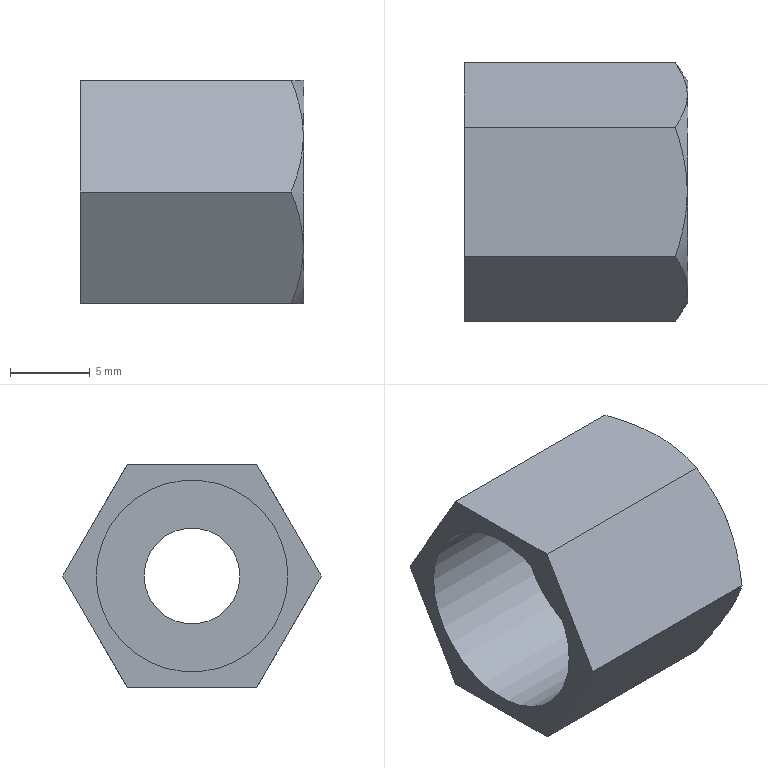Part | STEP file | 1-46.8 | 2 solids | 16 faces | box 14 x 16.166 x 14 mm | volume 1298 mm3 | plane 11 | cylinder 4 | cone 1 | commonest cylinder face diameters 6 x2 12 x2
STEP:
#1=CARTESIAN_POINT('',(0.,0.,0.));
#2=DIRECTION('',(0.,0.,1.));
#3=DIRECTION('',(1.,0.,0.));
#4=AXIS2_PLACEMENT_3D('',#1,#2,#3);
#5=CARTESIAN_POINT('',(11.,6.,0.));
#6=VERTEX_POINT('',#5);
#7=CARTESIAN_POINT('',(11.,0.,0.));
#8=DIRECTION('',(1.,0.,0.));
#9=DIRECTION('',(0.,1.,0.));
#10=AXIS2_PLACEMENT_3D('',#7,#8,#9);
#11=CIRCLE('',#10,6.);
#12=CARTESIAN_POINT('',(11.,-1.608,0.));
#13=DIRECTION('',(1.,0.,0.));
#14=DIRECTION('',(0.,0.,-1.));
#15=AXIS2_PLACEMENT_3D('',#12,#13,#14);
#16=PLANE('',#15);
#17=CARTESIAN_POINT('',(0.,1.608));
#18=DIRECTION('',(0.,1.));
#19=AXIS2_PLACEMENT_2D('',#17,#18);
#20=CIRCLE('',#19,6.);
#21=(GEOMETRIC_REPRESENTATION_CONTEXT(2)PARAMETRIC_REPRESENTATION_CONTEXT()REPRESENTATION_CONTEXT('',''));
#22=DEFINITIONAL_REPRESENTATION('',(#20),#21);
#23=PCURVE('',#16,#22);
#24=CARTESIAN_POINT('',(11.,0.,0.));
#25=DIRECTION('',(-1.,0.,0.));
#26=DIRECTION('',(0.,1.,0.));
#27=AXIS2_PLACEMENT_3D('',#24,#25,#26);
#28=CYLINDRICAL_SURFACE('',#27,6.);
#29=CARTESIAN_POINT('',(6.283,0.));
#30=DIRECTION('',(-1.,0.));
#31=VECTOR('',#30,1.);
#32=LINE('',#29,#31);
#33=(GEOMETRIC_REPRESENTATION_CONTEXT(2)PARAMETRIC_REPRESENTATION_CONTEXT()REPRESENTATION_CONTEXT('',''));
#34=DEFINITIONAL_REPRESENTATION('',(#32),#33);
#35=PCURVE('',#28,#34);
#36=SURFACE_CURVE('',#11,(#23,#35),.PCURVE_S1.);
#37=EDGE_CURVE('',#6,#6,#36,.T.);
#38=ORIENTED_EDGE('',*,*,#37,.T.);
#39=EDGE_LOOP('',(#38));
#40=FACE_BOUND('',#39,.T.);
#41=CARTESIAN_POINT('',(11.,3.,0.));
#42=VERTEX_POINT('',#41);
#43=CARTESIAN_POINT('',(11.,0.,0.));
#44=DIRECTION('',(-1.,0.,0.));
#45=DIRECTION('',(0.,1.,0.));
#46=AXIS2_PLACEMENT_3D('',#43,#44,#45);
#47=CIRCLE('',#46,3.);
#48=CARTESIAN_POINT('',(0.,4.608));
#49=CARTESIAN_POINT('',(5.196,4.608));
#50=CARTESIAN_POINT('',(2.598,0.1077));
#51=CARTESIAN_POINT('',(0.,-4.392));
#52=CARTESIAN_POINT('',(-2.598,0.1077));
#53=CARTESIAN_POINT('',(-5.196,4.608));
#54=CARTESIAN_POINT('',(0.,4.608));
#55=(BOUNDED_CURVE()B_SPLINE_CURVE(2,(#48,#49,#50,#51,#52,#53,#54),.UNSPECIFIED.,.T.,.F.)B_SPLINE_CURVE_WITH_KNOTS((1,2,2,2,2,1),(-2.094,0.,2.094,4.189,6.283,8.378),.UNSPECIFIED.)CURVE()GEOMETRIC_REPRESENTATION_ITEM()RATIONAL_B_SPLINE_CURVE((1.,0.5,1.,0.5,1.,0.5,1.))REPRESENTATION_ITEM(''));
#56=(GEOMETRIC_REPRESENTATION_CONTEXT(2)PARAMETRIC_REPRESENTATION_CONTEXT()REPRESENTATION_CONTEXT('',''));
#57=DEFINITIONAL_REPRESENTATION('',(#55),#56);
#58=PCURVE('',#16,#57);
#59=CARTESIAN_POINT('',(11.,0.,0.));
#60=DIRECTION('',(-1.,0.,0.));
#61=DIRECTION('',(0.,1.,0.));
#62=AXIS2_PLACEMENT_3D('',#59,#60,#61);
#63=CYLINDRICAL_SURFACE('',#62,3.);
#64=CARTESIAN_POINT('',(0.,0.));
#65=DIRECTION('',(1.,0.));
#66=VECTOR('',#65,1.);
#67=LINE('',#64,#66);
#68=(GEOMETRIC_REPRESENTATION_CONTEXT(2)PARAMETRIC_REPRESENTATION_CONTEXT()REPRESENTATION_CONTEXT('',''));
#69=DEFINITIONAL_REPRESENTATION('',(#67),#68);
#70=PCURVE('',#63,#69);
#71=SURFACE_CURVE('',#47,(#58,#70),.PCURVE_S1.);
#72=EDGE_CURVE('',#42,#42,#71,.T.);
#73=ORIENTED_EDGE('',*,*,#72,.T.);
#74=EDGE_LOOP('',(#73));
#75=FACE_BOUND('',#74,.T.);
#76=ADVANCED_FACE('',(#40,#75),#16,.T.);
#77=CARTESIAN_POINT('',(8.,6.,0.));
#78=VERTEX_POINT('',#77);
#79=CARTESIAN_POINT('',(8.,0.,0.));
#80=DIRECTION('',(1.,0.,0.));
#81=DIRECTION('',(0.,1.,0.));
#82=AXIS2_PLACEMENT_3D('',#79,#80,#81);
#83=CIRCLE('',#82,6.);
#84=CARTESIAN_POINT('',(8.,-1.608,0.));
#85=DIRECTION('',(1.,0.,0.));
#86=DIRECTION('',(0.,0.,-1.));
#87=AXIS2_PLACEMENT_3D('',#84,#85,#86);
#88=PLANE('',#87);
#89=CARTESIAN_POINT('',(0.,1.608));
#90=DIRECTION('',(0.,1.));
#91=AXIS2_PLACEMENT_2D('',#89,#90);
#92=CIRCLE('',#91,6.);
#93=(GEOMETRIC_REPRESENTATION_CONTEXT(2)PARAMETRIC_REPRESENTATION_CONTEXT()REPRESENTATION_CONTEXT('',''));
#94=DEFINITIONAL_REPRESENTATION('',(#92),#93);
#95=PCURVE('',#88,#94);
#96=CARTESIAN_POINT('',(6.283,3.));
#97=DIRECTION('',(-1.,0.));
#98=VECTOR('',#97,1.);
#99=LINE('',#96,#98);
#100=(GEOMETRIC_REPRESENTATION_CONTEXT(2)PARAMETRIC_REPRESENTATION_CONTEXT()REPRESENTATION_CONTEXT('',''));
#101=DEFINITIONAL_REPRESENTATION('',(#99),#100);
#102=PCURVE('',#28,#101);
#103=SURFACE_CURVE('',#83,(#95,#102),.PCURVE_S1.);
#104=EDGE_CURVE('',#78,#78,#103,.T.);
#105=ORIENTED_EDGE('',*,*,#104,.T.);
#106=EDGE_LOOP('',(#105));
#107=FACE_BOUND('',#106,.F.);
#108=CARTESIAN_POINT('',(8.,3.,0.));
#109=VERTEX_POINT('',#108);
#110=CARTESIAN_POINT('',(8.,0.,0.));
#111=DIRECTION('',(-1.,0.,0.));
#112=DIRECTION('',(0.,1.,0.));
#113=AXIS2_PLACEMENT_3D('',#110,#111,#112);
#114=CIRCLE('',#113,3.);
#115=CARTESIAN_POINT('',(0.,4.608));
#116=CARTESIAN_POINT('',(5.196,4.608));
#117=CARTESIAN_POINT('',(2.598,0.1077));
#118=CARTESIAN_POINT('',(0.,-4.392));
#119=CARTESIAN_POINT('',(-2.598,0.1077));
#120=CARTESIAN_POINT('',(-5.196,4.608));
#121=CARTESIAN_POINT('',(0.,4.608));
#122=(BOUNDED_CURVE()B_SPLINE_CURVE(2,(#115,#116,#117,#118,#119,#120,#121),.UNSPECIFIED.,.T.,.F.)B_SPLINE_CURVE_WITH_KNOTS((1,2,2,2,2,1),(-2.094,0.,2.094,4.189,6.283,8.378),.UNSPECIFIED.)CURVE()GEOMETRIC_REPRESENTATION_ITEM()RATIONAL_B_SPLINE_CURVE((1.,0.5,1.,0.5,1.,0.5,1.))REPRESENTATION_ITEM(''));
#123=(GEOMETRIC_REPRESENTATION_CONTEXT(2)PARAMETRIC_REPRESENTATION_CONTEXT()REPRESENTATION_CONTEXT('',''));
#124=DEFINITIONAL_REPRESENTATION('',(#122),#123);
#125=PCURVE('',#88,#124);
#126=CARTESIAN_POINT('',(0.,3.));
#127=DIRECTION('',(1.,0.));
#128=VECTOR('',#127,1.);
#129=LINE('',#126,#128);
#130=(GEOMETRIC_REPRESENTATION_CONTEXT(2)PARAMETRIC_REPRESENTATION_CONTEXT()REPRESENTATION_CONTEXT('',''));
#131=DEFINITIONAL_REPRESENTATION('',(#129),#130);
#132=PCURVE('',#63,#131);
#133=SURFACE_CURVE('',#114,(#125,#132),.PCURVE_S1.);
#134=EDGE_CURVE('',#109,#109,#133,.T.);
#135=ORIENTED_EDGE('',*,*,#134,.T.);
#136=EDGE_LOOP('',(#135));
#137=FACE_BOUND('',#136,.F.);
#138=ADVANCED_FACE('',(#107,#137),#88,.F.);
#139=CARTESIAN_POINT('',(11.,6.,0.));
#140=DIRECTION('',(-1.,0.,0.));
#141=VECTOR('',#140,1.);
#142=LINE('',#139,#141);
#143=CARTESIAN_POINT('',(6.283,0.));
#144=DIRECTION('',(0.,1.));
#145=VECTOR('',#144,1.);
#146=LINE('',#143,#145);
#147=(GEOMETRIC_REPRESENTATION_CONTEXT(2)PARAMETRIC_REPRESENTATION_CONTEXT()REPRESENTATION_CONTEXT('',''));
#148=DEFINITIONAL_REPRESENTATION('',(#146),#147);
#149=PCURVE('',#28,#148);
#150=CARTESIAN_POINT('',(0.,0.));
#151=DIRECTION('',(0.,1.));
#152=VECTOR('',#151,1.);
#153=LINE('',#150,#152);
#154=(GEOMETRIC_REPRESENTATION_CONTEXT(2)PARAMETRIC_REPRESENTATION_CONTEXT()REPRESENTATION_CONTEXT('',''));
#155=DEFINITIONAL_REPRESENTATION('',(#153),#154);
#156=PCURVE('',#28,#155);
#157=SEAM_CURVE('',#142,(#149,#156),.PCURVE_S1.);
#158=EDGE_CURVE('',#6,#78,#157,.T.);
#159=ORIENTED_EDGE('',*,*,#158,.T.);
#160=ORIENTED_EDGE('',*,*,#104,.T.);
#161=ORIENTED_EDGE('',*,*,#158,.F.);
#162=ORIENTED_EDGE('',*,*,#37,.F.);
#163=EDGE_LOOP('',(#159,#160,#161,#162));
#164=FACE_BOUND('',#163,.T.);
#165=ADVANCED_FACE('',(#164),#28,.T.);
#166=ORIENTED_EDGE('',*,*,#72,.T.);
#167=CARTESIAN_POINT('',(11.,3.,0.));
#168=DIRECTION('',(-1.,0.,0.));
#169=VECTOR('',#168,1.);
#170=LINE('',#167,#169);
#171=CARTESIAN_POINT('',(6.283,0.));
#172=DIRECTION('',(0.,1.));
#173=VECTOR('',#172,1.);
#174=LINE('',#171,#173);
#175=(GEOMETRIC_REPRESENTATION_CONTEXT(2)PARAMETRIC_REPRESENTATION_CONTEXT()REPRESENTATION_CONTEXT('',''));
#176=DEFINITIONAL_REPRESENTATION('',(#174),#175);
#177=PCURVE('',#63,#176);
#178=CARTESIAN_POINT('',(0.,0.));
#179=DIRECTION('',(0.,1.));
#180=VECTOR('',#179,1.);
#181=LINE('',#178,#180);
#182=(GEOMETRIC_REPRESENTATION_CONTEXT(2)PARAMETRIC_REPRESENTATION_CONTEXT()REPRESENTATION_CONTEXT('',''));
#183=DEFINITIONAL_REPRESENTATION('',(#181),#182);
#184=PCURVE('',#63,#183);
#185=SEAM_CURVE('',#170,(#177,#184),.PCURVE_S1.);
#186=EDGE_CURVE('',#42,#109,#185,.T.);
#187=ORIENTED_EDGE('',*,*,#186,.T.);
#188=ORIENTED_EDGE('',*,*,#134,.F.);
#189=ORIENTED_EDGE('',*,*,#186,.F.);
#190=EDGE_LOOP('',(#166,#187,#188,#189));
#191=FACE_BOUND('',#190,.F.);
#192=ADVANCED_FACE('',(#191),#63,.F.);
#193=CLOSED_SHELL('',(#76,#138,#165,#192));
#194=MANIFOLD_SOLID_BREP('',#193);
#195=CARTESIAN_POINT('',(0.,-4.041,7.));
#196=VERTEX_POINT('',#195);
#197=CARTESIAN_POINT('',(0.,4.041,7.));
#198=VERTEX_POINT('',#197);
#199=CARTESIAN_POINT('',(0.,-4.041,7.));
#200=DIRECTION('',(0.,1.,0.));
#201=VECTOR('',#200,1.);
#202=LINE('',#199,#201);
#203=CARTESIAN_POINT('',(0.,0.,1.083));
#204=DIRECTION('',(-1.,0.,0.));
#205=DIRECTION('',(0.,0.,1.));
#206=AXIS2_PLACEMENT_3D('',#203,#204,#205);
#207=PLANE('',#206);
#208=CARTESIAN_POINT('',(5.917,-4.041));
#209=DIRECTION('',(0.,1.));
#210=VECTOR('',#209,1.);
#211=LINE('',#208,#210);
#212=(GEOMETRIC_REPRESENTATION_CONTEXT(2)PARAMETRIC_REPRESENTATION_CONTEXT()REPRESENTATION_CONTEXT('',''));
#213=DEFINITIONAL_REPRESENTATION('',(#211),#212);
#214=PCURVE('',#207,#213);
#215=CARTESIAN_POINT('',(7.,0.,7.));
#216=DIRECTION('',(0.,0.,-1.));
#217=DIRECTION('',(0.,1.,0.));
#218=AXIS2_PLACEMENT_3D('',#215,#216,#217);
#219=PLANE('',#218);
#220=CARTESIAN_POINT('',(-4.041,-7.));
#221=DIRECTION('',(1.,0.));
#222=VECTOR('',#221,1.);
#223=LINE('',#220,#222);
#224=(GEOMETRIC_REPRESENTATION_CONTEXT(2)PARAMETRIC_REPRESENTATION_CONTEXT()REPRESENTATION_CONTEXT('',''));
#225=DEFINITIONAL_REPRESENTATION('',(#223),#224);
#226=PCURVE('',#219,#225);
#227=SURFACE_CURVE('',#202,(#214,#226),.PCURVE_S1.);
#228=EDGE_CURVE('',#196,#198,#227,.T.);
#229=ORIENTED_EDGE('',*,*,#228,.T.);
#230=CARTESIAN_POINT('',(0.,8.083,0.));
#231=VERTEX_POINT('',#230);
#232=CARTESIAN_POINT('',(0.,4.041,7.));
#233=DIRECTION('',(0.,0.5,-0.866));
#234=VECTOR('',#233,1.);
#235=LINE('',#232,#234);
#236=CARTESIAN_POINT('',(5.917,4.041));
#237=DIRECTION('',(-0.866,0.5));
#238=VECTOR('',#237,1.);
#239=LINE('',#236,#238);
#240=(GEOMETRIC_REPRESENTATION_CONTEXT(2)PARAMETRIC_REPRESENTATION_CONTEXT()REPRESENTATION_CONTEXT('',''));
#241=DEFINITIONAL_REPRESENTATION('',(#239),#240);
#242=PCURVE('',#207,#241);
#243=CARTESIAN_POINT('',(7.,6.062,3.5));
#244=DIRECTION('',(0.,-0.866,-0.5));
#245=DIRECTION('',(0.,0.5,-0.866));
#246=AXIS2_PLACEMENT_3D('',#243,#244,#245);
#247=PLANE('',#246);
#248=CARTESIAN_POINT('',(-4.041,-7.));
#249=DIRECTION('',(1.,0.));
#250=VECTOR('',#249,1.);
#251=LINE('',#248,#250);
#252=(GEOMETRIC_REPRESENTATION_CONTEXT(2)PARAMETRIC_REPRESENTATION_CONTEXT()REPRESENTATION_CONTEXT('',''));
#253=DEFINITIONAL_REPRESENTATION('',(#251),#252);
#254=PCURVE('',#247,#253);
#255=SURFACE_CURVE('',#235,(#242,#254),.PCURVE_S1.);
#256=EDGE_CURVE('',#198,#231,#255,.T.);
#257=ORIENTED_EDGE('',*,*,#256,.T.);
#258=CARTESIAN_POINT('',(0.,4.041,-7.));
#259=VERTEX_POINT('',#258);
#260=CARTESIAN_POINT('',(0.,8.083,0.));
#261=DIRECTION('',(0.,-0.5,-0.866));
#262=VECTOR('',#261,1.);
#263=LINE('',#260,#262);
#264=CARTESIAN_POINT('',(-1.083,8.083));
#265=DIRECTION('',(-0.866,-0.5));
#266=VECTOR('',#265,1.);
#267=LINE('',#264,#266);
#268=(GEOMETRIC_REPRESENTATION_CONTEXT(2)PARAMETRIC_REPRESENTATION_CONTEXT()REPRESENTATION_CONTEXT('',''));
#269=DEFINITIONAL_REPRESENTATION('',(#267),#268);
#270=PCURVE('',#207,#269);
#271=CARTESIAN_POINT('',(7.,6.062,-3.5));
#272=DIRECTION('',(0.,-0.866,0.5));
#273=DIRECTION('',(0.,-0.5,-0.866));
#274=AXIS2_PLACEMENT_3D('',#271,#272,#273);
#275=PLANE('',#274);
#276=CARTESIAN_POINT('',(-4.041,-7.));
#277=DIRECTION('',(1.,0.));
#278=VECTOR('',#277,1.);
#279=LINE('',#276,#278);
#280=(GEOMETRIC_REPRESENTATION_CONTEXT(2)PARAMETRIC_REPRESENTATION_CONTEXT()REPRESENTATION_CONTEXT('',''));
#281=DEFINITIONAL_REPRESENTATION('',(#279),#280);
#282=PCURVE('',#275,#281);
#283=SURFACE_CURVE('',#263,(#270,#282),.PCURVE_S1.);
#284=EDGE_CURVE('',#231,#259,#283,.T.);
#285=ORIENTED_EDGE('',*,*,#284,.T.);
#286=CARTESIAN_POINT('',(0.,-4.041,-7.));
#287=VERTEX_POINT('',#286);
#288=CARTESIAN_POINT('',(0.,4.041,-7.));
#289=DIRECTION('',(0.,-1.,0.));
#290=VECTOR('',#289,1.);
#291=LINE('',#288,#290);
#292=CARTESIAN_POINT('',(-8.083,4.041));
#293=DIRECTION('',(0.,-1.));
#294=VECTOR('',#293,1.);
#295=LINE('',#292,#294);
#296=(GEOMETRIC_REPRESENTATION_CONTEXT(2)PARAMETRIC_REPRESENTATION_CONTEXT()REPRESENTATION_CONTEXT('',''));
#297=DEFINITIONAL_REPRESENTATION('',(#295),#296);
#298=PCURVE('',#207,#297);
#299=CARTESIAN_POINT('',(7.,0.,-7.));
#300=DIRECTION('',(0.,0.,1.));
#301=DIRECTION('',(0.,-1.,0.));
#302=AXIS2_PLACEMENT_3D('',#299,#300,#301);
#303=PLANE('',#302);
#304=CARTESIAN_POINT('',(-4.041,-7.));
#305=DIRECTION('',(1.,0.));
#306=VECTOR('',#305,1.);
#307=LINE('',#304,#306);
#308=(GEOMETRIC_REPRESENTATION_CONTEXT(2)PARAMETRIC_REPRESENTATION_CONTEXT()REPRESENTATION_CONTEXT('',''));
#309=DEFINITIONAL_REPRESENTATION('',(#307),#308);
#310=PCURVE('',#303,#309);
#311=SURFACE_CURVE('',#291,(#298,#310),.PCURVE_S1.);
#312=EDGE_CURVE('',#259,#287,#311,.T.);
#313=ORIENTED_EDGE('',*,*,#312,.T.);
#314=CARTESIAN_POINT('',(0.,-8.083,0.));
#315=VERTEX_POINT('',#314);
#316=CARTESIAN_POINT('',(0.,-4.041,-7.));
#317=DIRECTION('',(0.,-0.5,0.866));
#318=VECTOR('',#317,1.);
#319=LINE('',#316,#318);
#320=CARTESIAN_POINT('',(-8.083,-4.041));
#321=DIRECTION('',(0.866,-0.5));
#322=VECTOR('',#321,1.);
#323=LINE('',#320,#322);
#324=(GEOMETRIC_REPRESENTATION_CONTEXT(2)PARAMETRIC_REPRESENTATION_CONTEXT()REPRESENTATION_CONTEXT('',''));
#325=DEFINITIONAL_REPRESENTATION('',(#323),#324);
#326=PCURVE('',#207,#325);
#327=CARTESIAN_POINT('',(7.,-6.062,-3.5));
#328=DIRECTION('',(0.,0.866,0.5));
#329=DIRECTION('',(0.,-0.5,0.866));
#330=AXIS2_PLACEMENT_3D('',#327,#328,#329);
#331=PLANE('',#330);
#332=CARTESIAN_POINT('',(-4.041,-7.));
#333=DIRECTION('',(1.,0.));
#334=VECTOR('',#333,1.);
#335=LINE('',#332,#334);
#336=(GEOMETRIC_REPRESENTATION_CONTEXT(2)PARAMETRIC_REPRESENTATION_CONTEXT()REPRESENTATION_CONTEXT('',''));
#337=DEFINITIONAL_REPRESENTATION('',(#335),#336);
#338=PCURVE('',#331,#337);
#339=SURFACE_CURVE('',#319,(#326,#338),.PCURVE_S1.);
#340=EDGE_CURVE('',#287,#315,#339,.T.);
#341=ORIENTED_EDGE('',*,*,#340,.T.);
#342=CARTESIAN_POINT('',(0.,-8.083,0.));
#343=DIRECTION('',(0.,0.5,0.866));
#344=VECTOR('',#343,1.);
#345=LINE('',#342,#344);
#346=CARTESIAN_POINT('',(-1.083,-8.083));
#347=DIRECTION('',(0.866,0.5));
#348=VECTOR('',#347,1.);
#349=LINE('',#346,#348);
#350=(GEOMETRIC_REPRESENTATION_CONTEXT(2)PARAMETRIC_REPRESENTATION_CONTEXT()REPRESENTATION_CONTEXT('',''));
#351=DEFINITIONAL_REPRESENTATION('',(#349),#350);
#352=PCURVE('',#207,#351);
#353=CARTESIAN_POINT('',(7.,-6.062,3.5));
#354=DIRECTION('',(0.,0.866,-0.5));
#355=DIRECTION('',(0.,0.5,0.866));
#356=AXIS2_PLACEMENT_3D('',#353,#354,#355);
#357=PLANE('',#356);
#358=CARTESIAN_POINT('',(-4.041,-7.));
#359=DIRECTION('',(1.,0.));
#360=VECTOR('',#359,1.);
#361=LINE('',#358,#360);
#362=(GEOMETRIC_REPRESENTATION_CONTEXT(2)PARAMETRIC_REPRESENTATION_CONTEXT()REPRESENTATION_CONTEXT('',''));
#363=DEFINITIONAL_REPRESENTATION('',(#361),#362);
#364=PCURVE('',#357,#363);
#365=SURFACE_CURVE('',#345,(#352,#364),.PCURVE_S1.);
#366=EDGE_CURVE('',#315,#196,#365,.T.);
#367=ORIENTED_EDGE('',*,*,#366,.T.);
#368=EDGE_LOOP('',(#229,#257,#285,#313,#341,#367));
#369=FACE_BOUND('',#368,.T.);
#370=CARTESIAN_POINT('',(0.,6.,0.));
#371=VERTEX_POINT('',#370);
#372=CARTESIAN_POINT('',(0.,0.,0.));
#373=DIRECTION('',(1.,0.,0.));
#374=DIRECTION('',(0.,1.,0.));
#375=AXIS2_PLACEMENT_3D('',#372,#373,#374);
#376=CIRCLE('',#375,6.);
#377=CARTESIAN_POINT('',(-1.083,6.));
#378=CARTESIAN_POINT('',(9.309,6.));
#379=CARTESIAN_POINT('',(4.113,-3.));
#380=CARTESIAN_POINT('',(-1.083,-12.));
#381=CARTESIAN_POINT('',(-6.279,-3.));
#382=CARTESIAN_POINT('',(-11.475,6.));
#383=CARTESIAN_POINT('',(-1.083,6.));
#384=(BOUNDED_CURVE()B_SPLINE_CURVE(2,(#377,#378,#379,#380,#381,#382,#383),.UNSPECIFIED.,.T.,.F.)B_SPLINE_CURVE_WITH_KNOTS((1,2,2,2,2,1),(-2.094,0.,2.094,4.189,6.283,8.378),.UNSPECIFIED.)CURVE()GEOMETRIC_REPRESENTATION_ITEM()RATIONAL_B_SPLINE_CURVE((1.,0.5,1.,0.5,1.,0.5,1.))REPRESENTATION_ITEM(''));
#385=(GEOMETRIC_REPRESENTATION_CONTEXT(2)PARAMETRIC_REPRESENTATION_CONTEXT()REPRESENTATION_CONTEXT('',''));
#386=DEFINITIONAL_REPRESENTATION('',(#384),#385);
#387=PCURVE('',#207,#386);
#388=CARTESIAN_POINT('',(0.,0.,0.));
#389=DIRECTION('',(1.,0.,0.));
#390=DIRECTION('',(0.,1.,0.));
#391=AXIS2_PLACEMENT_3D('',#388,#389,#390);
#392=CYLINDRICAL_SURFACE('',#391,6.);
#393=CARTESIAN_POINT('',(0.,0.));
#394=DIRECTION('',(1.,0.));
#395=VECTOR('',#394,1.);
#396=LINE('',#393,#395);
#397=(GEOMETRIC_REPRESENTATION_CONTEXT(2)PARAMETRIC_REPRESENTATION_CONTEXT()REPRESENTATION_CONTEXT('',''));
#398=DEFINITIONAL_REPRESENTATION('',(#396),#397);
#399=PCURVE('',#392,#398);
#400=SURFACE_CURVE('',#376,(#387,#399),.PCURVE_S1.);
#401=EDGE_CURVE('',#371,#371,#400,.T.);
#402=ORIENTED_EDGE('',*,*,#401,.T.);
#403=EDGE_LOOP('',(#402));
#404=FACE_BOUND('',#403,.T.);
#405=ADVANCED_FACE('',(#369,#404),#207,.T.);
#406=ORIENTED_EDGE('',*,*,#401,.T.);
#407=CARTESIAN_POINT('',(11.,6.,0.));
#408=VERTEX_POINT('',#407);
#409=CARTESIAN_POINT('',(0.,6.,0.));
#410=DIRECTION('',(1.,0.,0.));
#411=VECTOR('',#410,1.);
#412=LINE('',#409,#411);
#413=CARTESIAN_POINT('',(6.283,0.));
#414=DIRECTION('',(0.,1.));
#415=VECTOR('',#414,1.);
#416=LINE('',#413,#415);
#417=(GEOMETRIC_REPRESENTATION_CONTEXT(2)PARAMETRIC_REPRESENTATION_CONTEXT()REPRESENTATION_CONTEXT('',''));
#418=DEFINITIONAL_REPRESENTATION('',(#416),#417);
#419=PCURVE('',#392,#418);
#420=CARTESIAN_POINT('',(0.,0.));
#421=DIRECTION('',(0.,1.));
#422=VECTOR('',#421,1.);
#423=LINE('',#420,#422);
#424=(GEOMETRIC_REPRESENTATION_CONTEXT(2)PARAMETRIC_REPRESENTATION_CONTEXT()REPRESENTATION_CONTEXT('',''));
#425=DEFINITIONAL_REPRESENTATION('',(#423),#424);
#426=PCURVE('',#392,#425);
#427=SEAM_CURVE('',#412,(#419,#426),.PCURVE_S1.);
#428=EDGE_CURVE('',#371,#408,#427,.T.);
#429=ORIENTED_EDGE('',*,*,#428,.T.);
#430=CARTESIAN_POINT('',(11.,0.,0.));
#431=DIRECTION('',(1.,0.,0.));
#432=DIRECTION('',(0.,1.,0.));
#433=AXIS2_PLACEMENT_3D('',#430,#431,#432);
#434=CIRCLE('',#433,6.);
#435=CARTESIAN_POINT('',(0.,11.));
#436=DIRECTION('',(1.,0.));
#437=VECTOR('',#436,1.);
#438=LINE('',#435,#437);
#439=(GEOMETRIC_REPRESENTATION_CONTEXT(2)PARAMETRIC_REPRESENTATION_CONTEXT()REPRESENTATION_CONTEXT('',''));
#440=DEFINITIONAL_REPRESENTATION('',(#438),#439);
#441=PCURVE('',#392,#440);
#442=CARTESIAN_POINT('',(11.,-1.608,0.));
#443=DIRECTION('',(1.,0.,0.));
#444=DIRECTION('',(0.,0.,-1.));
#445=AXIS2_PLACEMENT_3D('',#442,#443,#444);
#446=PLANE('',#445);
#447=CARTESIAN_POINT('',(0.,1.608));
#448=DIRECTION('',(0.,1.));
#449=AXIS2_PLACEMENT_2D('',#447,#448);
#450=CIRCLE('',#449,6.);
#451=(GEOMETRIC_REPRESENTATION_CONTEXT(2)PARAMETRIC_REPRESENTATION_CONTEXT()REPRESENTATION_CONTEXT('',''));
#452=DEFINITIONAL_REPRESENTATION('',(#450),#451);
#453=PCURVE('',#446,#452);
#454=SURFACE_CURVE('',#434,(#441,#453),.PCURVE_S1.);
#455=EDGE_CURVE('',#408,#408,#454,.T.);
#456=ORIENTED_EDGE('',*,*,#455,.F.);
#457=ORIENTED_EDGE('',*,*,#428,.F.);
#458=EDGE_LOOP('',(#406,#429,#456,#457));
#459=FACE_BOUND('',#458,.F.);
#460=ADVANCED_FACE('',(#459),#392,.F.);
#461=ORIENTED_EDGE('',*,*,#455,.T.);
#462=EDGE_LOOP('',(#461));
#463=FACE_BOUND('',#462,.F.);
#464=CARTESIAN_POINT('',(11.,3.,0.));
#465=VERTEX_POINT('',#464);
#466=CARTESIAN_POINT('',(11.,0.,0.));
#467=DIRECTION('',(-1.,0.,0.));
#468=DIRECTION('',(0.,1.,0.));
#469=AXIS2_PLACEMENT_3D('',#466,#467,#468);
#470=CIRCLE('',#469,3.);
#471=CARTESIAN_POINT('',(0.,4.608));
#472=CARTESIAN_POINT('',(5.196,4.608));
#473=CARTESIAN_POINT('',(2.598,0.1077));
#474=CARTESIAN_POINT('',(0.,-4.392));
#475=CARTESIAN_POINT('',(-2.598,0.1077));
#476=CARTESIAN_POINT('',(-5.196,4.608));
#477=CARTESIAN_POINT('',(0.,4.608));
#478=(BOUNDED_CURVE()B_SPLINE_CURVE(2,(#471,#472,#473,#474,#475,#476,#477),.UNSPECIFIED.,.T.,.F.)B_SPLINE_CURVE_WITH_KNOTS((1,2,2,2,2,1),(-2.094,0.,2.094,4.189,6.283,8.378),.UNSPECIFIED.)CURVE()GEOMETRIC_REPRESENTATION_ITEM()RATIONAL_B_SPLINE_CURVE((1.,0.5,1.,0.5,1.,0.5,1.))REPRESENTATION_ITEM(''));
#479=(GEOMETRIC_REPRESENTATION_CONTEXT(2)PARAMETRIC_REPRESENTATION_CONTEXT()REPRESENTATION_CONTEXT('',''));
#480=DEFINITIONAL_REPRESENTATION('',(#478),#479);
#481=PCURVE('',#446,#480);
#482=CARTESIAN_POINT('',(0.,0.,0.));
#483=DIRECTION('',(1.,0.,0.));
#484=DIRECTION('',(0.,1.,0.));
#485=AXIS2_PLACEMENT_3D('',#482,#483,#484);
#486=CYLINDRICAL_SURFACE('',#485,3.);
#487=CARTESIAN_POINT('',(6.283,11.));
#488=DIRECTION('',(-1.,0.));
#489=VECTOR('',#488,1.);
#490=LINE('',#487,#489);
#491=(GEOMETRIC_REPRESENTATION_CONTEXT(2)PARAMETRIC_REPRESENTATION_CONTEXT()REPRESENTATION_CONTEXT('',''));
#492=DEFINITIONAL_REPRESENTATION('',(#490),#491);
#493=PCURVE('',#486,#492);
#494=SURFACE_CURVE('',#470,(#481,#493),.PCURVE_S1.);
#495=EDGE_CURVE('',#465,#465,#494,.T.);
#496=ORIENTED_EDGE('',*,*,#495,.T.);
#497=EDGE_LOOP('',(#496));
#498=FACE_BOUND('',#497,.F.);
#499=ADVANCED_FACE('',(#463,#498),#446,.F.);
#500=CARTESIAN_POINT('',(14.,3.,0.));
#501=VERTEX_POINT('',#500);
#502=CARTESIAN_POINT('',(14.,0.,0.));
#503=DIRECTION('',(1.,0.,0.));
#504=DIRECTION('',(0.,1.,0.));
#505=AXIS2_PLACEMENT_3D('',#502,#503,#504);
#506=CIRCLE('',#505,3.);
#507=CARTESIAN_POINT('',(0.,14.));
#508=DIRECTION('',(1.,0.));
#509=VECTOR('',#508,1.);
#510=LINE('',#507,#509);
#511=(GEOMETRIC_REPRESENTATION_CONTEXT(2)PARAMETRIC_REPRESENTATION_CONTEXT()REPRESENTATION_CONTEXT('',''));
#512=DEFINITIONAL_REPRESENTATION('',(#510),#511);
#513=PCURVE('',#486,#512);
#514=CARTESIAN_POINT('',(14.,0.,1.083));
#515=DIRECTION('',(-1.,0.,0.));
#516=DIRECTION('',(0.,0.,1.));
#517=AXIS2_PLACEMENT_3D('',#514,#515,#516);
#518=PLANE('',#517);
#519=CARTESIAN_POINT('',(-1.083,3.));
#520=CARTESIAN_POINT('',(4.113,3.));
#521=CARTESIAN_POINT('',(1.515,-1.5));
#522=CARTESIAN_POINT('',(-1.083,-6.));
#523=CARTESIAN_POINT('',(-3.681,-1.5));
#524=CARTESIAN_POINT('',(-6.279,3.));
#525=CARTESIAN_POINT('',(-1.083,3.));
#526=(BOUNDED_CURVE()B_SPLINE_CURVE(2,(#519,#520,#521,#522,#523,#524,#525),.UNSPECIFIED.,.T.,.F.)B_SPLINE_CURVE_WITH_KNOTS((1,2,2,2,2,1),(-2.094,0.,2.094,4.189,6.283,8.378),.UNSPECIFIED.)CURVE()GEOMETRIC_REPRESENTATION_ITEM()RATIONAL_B_SPLINE_CURVE((1.,0.5,1.,0.5,1.,0.5,1.))REPRESENTATION_ITEM(''));
#527=(GEOMETRIC_REPRESENTATION_CONTEXT(2)PARAMETRIC_REPRESENTATION_CONTEXT()REPRESENTATION_CONTEXT('',''));
#528=DEFINITIONAL_REPRESENTATION('',(#526),#527);
#529=PCURVE('',#518,#528);
#530=SURFACE_CURVE('',#506,(#513,#529),.PCURVE_S1.);
#531=EDGE_CURVE('',#501,#501,#530,.T.);
#532=ORIENTED_EDGE('',*,*,#531,.F.);
#533=CARTESIAN_POINT('',(11.,3.,0.));
#534=DIRECTION('',(1.,0.,0.));
#535=VECTOR('',#534,1.);
#536=LINE('',#533,#535);
#537=CARTESIAN_POINT('',(0.,11.));
#538=DIRECTION('',(0.,1.));
#539=VECTOR('',#538,1.);
#540=LINE('',#537,#539);
#541=(GEOMETRIC_REPRESENTATION_CONTEXT(2)PARAMETRIC_REPRESENTATION_CONTEXT()REPRESENTATION_CONTEXT('',''));
#542=DEFINITIONAL_REPRESENTATION('',(#540),#541);
#543=PCURVE('',#486,#542);
#544=CARTESIAN_POINT('',(6.283,11.));
#545=DIRECTION('',(0.,1.));
#546=VECTOR('',#545,1.);
#547=LINE('',#544,#546);
#548=(GEOMETRIC_REPRESENTATION_CONTEXT(2)PARAMETRIC_REPRESENTATION_CONTEXT()REPRESENTATION_CONTEXT('',''));
#549=DEFINITIONAL_REPRESENTATION('',(#547),#548);
#550=PCURVE('',#486,#549);
#551=SEAM_CURVE('',#536,(#543,#550),.PCURVE_S1.);
#552=EDGE_CURVE('',#465,#501,#551,.T.);
#553=ORIENTED_EDGE('',*,*,#552,.F.);
#554=ORIENTED_EDGE('',*,*,#495,.F.);
#555=ORIENTED_EDGE('',*,*,#552,.T.);
#556=EDGE_LOOP('',(#532,#553,#554,#555));
#557=FACE_BOUND('',#556,.F.);
#558=ADVANCED_FACE('',(#557),#486,.F.);
#559=ORIENTED_EDGE('',*,*,#228,.T.);
#560=CARTESIAN_POINT('',(13.208,4.041,7.));
#561=VERTEX_POINT('',#560);
#562=CARTESIAN_POINT('',(0.,4.041,7.));
#563=DIRECTION('',(1.,0.,0.));
#564=VECTOR('',#563,1.);
#565=LINE('',#562,#564);
#566=CARTESIAN_POINT('',(4.041,-7.));
#567=DIRECTION('',(0.,1.));
#568=VECTOR('',#567,1.);
#569=LINE('',#566,#568);
#570=(GEOMETRIC_REPRESENTATION_CONTEXT(2)PARAMETRIC_REPRESENTATION_CONTEXT()REPRESENTATION_CONTEXT('',''));
#571=DEFINITIONAL_REPRESENTATION('',(#569),#570);
#572=PCURVE('',#219,#571);
#573=CARTESIAN_POINT('',(-4.041,-7.));
#574=DIRECTION('',(0.,1.));
#575=VECTOR('',#574,1.);
#576=LINE('',#573,#575);
#577=(GEOMETRIC_REPRESENTATION_CONTEXT(2)PARAMETRIC_REPRESENTATION_CONTEXT()REPRESENTATION_CONTEXT('',''));
#578=DEFINITIONAL_REPRESENTATION('',(#576),#577);
#579=PCURVE('',#247,#578);
#580=SURFACE_CURVE('',#565,(#572,#579),.PCURVE_S1.);
#581=EDGE_CURVE('',#198,#561,#580,.T.);
#582=ORIENTED_EDGE('',*,*,#581,.T.);
#583=CARTESIAN_POINT('',(13.955,0.,7.));
#584=VERTEX_POINT('',#583);
#585=CARTESIAN_POINT('',(13.208,4.041,7.));
#586=CARTESIAN_POINT('',(13.955,1.876,7.));
#587=CARTESIAN_POINT('',(13.955,0.,7.));
#588=(BOUNDED_CURVE()B_SPLINE_CURVE(2,(#585,#586,#587),.UNSPECIFIED.,.F.,.F.)B_SPLINE_CURVE_WITH_KNOTS((3,3),(0.,1.),.PIECEWISE_BEZIER_KNOTS.)CURVE()GEOMETRIC_REPRESENTATION_ITEM()RATIONAL_B_SPLINE_CURVE((1.524,1.642,1.642))REPRESENTATION_ITEM(''));
#589=CARTESIAN_POINT('',(4.041,6.208));
#590=CARTESIAN_POINT('',(1.876,6.955));
#591=CARTESIAN_POINT('',(0.,6.955));
#592=(BOUNDED_CURVE()B_SPLINE_CURVE(2,(#589,#590,#591),.UNSPECIFIED.,.F.,.F.)B_SPLINE_CURVE_WITH_KNOTS((3,3),(0.,1.),.PIECEWISE_BEZIER_KNOTS.)CURVE()GEOMETRIC_REPRESENTATION_ITEM()RATIONAL_B_SPLINE_CURVE((1.524,1.642,1.642))REPRESENTATION_ITEM(''));
#593=(GEOMETRIC_REPRESENTATION_CONTEXT(2)PARAMETRIC_REPRESENTATION_CONTEXT()REPRESENTATION_CONTEXT('',''));
#594=DEFINITIONAL_REPRESENTATION('',(#592),#593);
#595=PCURVE('',#219,#594);
#596=CARTESIAN_POINT('',(14.,0.,0.));
#597=DIRECTION('',(-1.,0.,0.));
#598=DIRECTION('',(0.,0.,1.));
#599=AXIS2_PLACEMENT_3D('',#596,#597,#598);
#600=CONICAL_SURFACE('',#599,6.935,0.9667);
#601=CARTESIAN_POINT('',(0.5236,0.792));
#602=CARTESIAN_POINT('',(0.516,0.7676));
#603=CARTESIAN_POINT('',(0.5008,0.7203));
#604=CARTESIAN_POINT('',(0.4779,0.6535));
#605=CARTESIAN_POINT('',(0.4548,0.5907));
#606=CARTESIAN_POINT('',(0.4317,0.5319));
#607=CARTESIAN_POINT('',(0.4084,0.4768));
#608=CARTESIAN_POINT('',(0.3849,0.4255));
#609=CARTESIAN_POINT('',(0.3614,0.3777));
#610=CARTESIAN_POINT('',(0.3378,0.3334));
#611=CARTESIAN_POINT('',(0.3141,0.2926));
#612=CARTESIAN_POINT('',(0.2903,0.255));
#613=CARTESIAN_POINT('',(0.2664,0.2207));
#614=CARTESIAN_POINT('',(0.2424,0.1896));
#615=CARTESIAN_POINT('',(0.2184,0.1617));
#616=CARTESIAN_POINT('',(0.1943,0.1368));
#617=CARTESIAN_POINT('',(0.1701,0.1149));
#618=CARTESIAN_POINT('',(0.1459,0.09605));
#619=CARTESIAN_POINT('',(0.1217,0.08014));
#620=CARTESIAN_POINT('',(0.09736,0.06717));
#621=CARTESIAN_POINT('',(0.07305,0.0571));
#622=CARTESIAN_POINT('',(0.04871,0.04992));
#623=CARTESIAN_POINT('',(0.02436,0.04562));
#624=CARTESIAN_POINT('',(0.00812,0.04466));
#625=CARTESIAN_POINT('',(0.,0.04466));
#626=B_SPLINE_CURVE_WITH_KNOTS('',3,(#601,#602,#603,#604,#605,#606,#607,#608,#609,#610,#611,#612,#613,#614,#615,#616,#617,#618,#619,#620,#621,#622,#623,#624,#625),.UNSPECIFIED.,.F.,.F.,(4,1,1,1,1,1,1,1,1,1,1,1,1,1,1,1,1,1,1,1,1,1,4),(0.,0.04545,0.09091,0.1364,0.1818,0.2273,0.2727,0.3182,0.3636,0.4091,0.4545,0.5,0.5455,0.5909,0.6364,0.6818,0.7273,0.7727,0.8182,0.8636,0.9091,0.9545,1.),.QUASI_UNIFORM_KNOTS.);
#627=(GEOMETRIC_REPRESENTATION_CONTEXT(2)PARAMETRIC_REPRESENTATION_CONTEXT()REPRESENTATION_CONTEXT('',''));
#628=DEFINITIONAL_REPRESENTATION('',(#626),#627);
#629=PCURVE('',#600,#628);
#630=SURFACE_CURVE('',#588,(#595,#629),.PCURVE_S1.);
#631=EDGE_CURVE('',#561,#584,#630,.T.);
#632=ORIENTED_EDGE('',*,*,#631,.T.);
#633=CARTESIAN_POINT('',(13.208,-4.041,7.));
#634=VERTEX_POINT('',#633);
#635=CARTESIAN_POINT('',(13.955,0.,7.));
#636=CARTESIAN_POINT('',(13.955,-1.876,7.));
#637=CARTESIAN_POINT('',(13.208,-4.041,7.));
#638=(BOUNDED_CURVE()B_SPLINE_CURVE(2,(#635,#636,#637),.UNSPECIFIED.,.F.,.F.)B_SPLINE_CURVE_WITH_KNOTS((3,3),(0.,1.),.PIECEWISE_BEZIER_KNOTS.)CURVE()GEOMETRIC_REPRESENTATION_ITEM()RATIONAL_B_SPLINE_CURVE((1.642,1.642,1.524))REPRESENTATION_ITEM(''));
#639=CARTESIAN_POINT('',(0.,6.955));
#640=CARTESIAN_POINT('',(-1.876,6.955));
#641=CARTESIAN_POINT('',(-4.041,6.208));
#642=(BOUNDED_CURVE()B_SPLINE_CURVE(2,(#639,#640,#641),.UNSPECIFIED.,.F.,.F.)B_SPLINE_CURVE_WITH_KNOTS((3,3),(0.,1.),.PIECEWISE_BEZIER_KNOTS.)CURVE()GEOMETRIC_REPRESENTATION_ITEM()RATIONAL_B_SPLINE_CURVE((1.642,1.642,1.524))REPRESENTATION_ITEM(''));
#643=(GEOMETRIC_REPRESENTATION_CONTEXT(2)PARAMETRIC_REPRESENTATION_CONTEXT()REPRESENTATION_CONTEXT('',''));
#644=DEFINITIONAL_REPRESENTATION('',(#642),#643);
#645=PCURVE('',#219,#644);
#646=CARTESIAN_POINT('',(6.283,0.04466));
#647=CARTESIAN_POINT('',(6.275,0.04466));
#648=CARTESIAN_POINT('',(6.259,0.04562));
#649=CARTESIAN_POINT('',(6.234,0.04992));
#650=CARTESIAN_POINT('',(6.21,0.0571));
#651=CARTESIAN_POINT('',(6.186,0.06717));
#652=CARTESIAN_POINT('',(6.162,0.08014));
#653=CARTESIAN_POINT('',(6.137,0.09605));
#654=CARTESIAN_POINT('',(6.113,0.1149));
#655=CARTESIAN_POINT('',(6.089,0.1368));
#656=CARTESIAN_POINT('',(6.065,0.1617));
#657=CARTESIAN_POINT('',(6.041,0.1896));
#658=CARTESIAN_POINT('',(6.017,0.2207));
#659=CARTESIAN_POINT('',(5.993,0.255));
#660=CARTESIAN_POINT('',(5.969,0.2926));
#661=CARTESIAN_POINT('',(5.945,0.3334));
#662=CARTESIAN_POINT('',(5.922,0.3777));
#663=CARTESIAN_POINT('',(5.898,0.4255));
#664=CARTESIAN_POINT('',(5.875,0.4768));
#665=CARTESIAN_POINT('',(5.852,0.5319));
#666=CARTESIAN_POINT('',(5.828,0.5907));
#667=CARTESIAN_POINT('',(5.805,0.6535));
#668=CARTESIAN_POINT('',(5.782,0.7203));
#669=CARTESIAN_POINT('',(5.767,0.7676));
#670=CARTESIAN_POINT('',(5.76,0.792));
#671=B_SPLINE_CURVE_WITH_KNOTS('',3,(#646,#647,#648,#649,#650,#651,#652,#653,#654,#655,#656,#657,#658,#659,#660,#661,#662,#663,#664,#665,#666,#667,#668,#669,#670),.UNSPECIFIED.,.F.,.F.,(4,1,1,1,1,1,1,1,1,1,1,1,1,1,1,1,1,1,1,1,1,1,4),(0.,0.04545,0.09091,0.1364,0.1818,0.2273,0.2727,0.3182,0.3636,0.4091,0.4545,0.5,0.5455,0.5909,0.6364,0.6818,0.7273,0.7727,0.8182,0.8636,0.9091,0.9545,1.),.QUASI_UNIFORM_KNOTS.);
#672=(GEOMETRIC_REPRESENTATION_CONTEXT(2)PARAMETRIC_REPRESENTATION_CONTEXT()REPRESENTATION_CONTEXT('',''));
#673=DEFINITIONAL_REPRESENTATION('',(#671),#672);
#674=PCURVE('',#600,#673);
#675=SURFACE_CURVE('',#638,(#645,#674),.PCURVE_S1.);
#676=EDGE_CURVE('',#584,#634,#675,.T.);
#677=ORIENTED_EDGE('',*,*,#676,.T.);
#678=CARTESIAN_POINT('',(0.,-4.041,7.));
#679=DIRECTION('',(1.,0.,0.));
#680=VECTOR('',#679,1.);
#681=LINE('',#678,#680);
#682=CARTESIAN_POINT('',(-4.041,-7.));
#683=DIRECTION('',(0.,1.));
#684=VECTOR('',#683,1.);
#685=LINE('',#682,#684);
#686=(GEOMETRIC_REPRESENTATION_CONTEXT(2)PARAMETRIC_REPRESENTATION_CONTEXT()REPRESENTATION_CONTEXT('',''));
#687=DEFINITIONAL_REPRESENTATION('',(#685),#686);
#688=PCURVE('',#219,#687);
#689=CARTESIAN_POINT('',(4.041,-7.));
#690=DIRECTION('',(0.,1.));
#691=VECTOR('',#690,1.);
#692=LINE('',#689,#691);
#693=(GEOMETRIC_REPRESENTATION_CONTEXT(2)PARAMETRIC_REPRESENTATION_CONTEXT()REPRESENTATION_CONTEXT('',''));
#694=DEFINITIONAL_REPRESENTATION('',(#692),#693);
#695=PCURVE('',#357,#694);
#696=SURFACE_CURVE('',#681,(#688,#695),.PCURVE_S1.);
#697=EDGE_CURVE('',#196,#634,#696,.T.);
#698=ORIENTED_EDGE('',*,*,#697,.F.);
#699=EDGE_LOOP('',(#559,#582,#632,#677,#698));
#700=FACE_BOUND('',#699,.F.);
#701=ADVANCED_FACE('',(#700),#219,.F.);
#702=ORIENTED_EDGE('',*,*,#256,.T.);
#703=CARTESIAN_POINT('',(13.208,8.083,0.));
#704=VERTEX_POINT('',#703);
#705=CARTESIAN_POINT('',(0.,8.083,0.));
#706=DIRECTION('',(1.,0.,0.));
#707=VECTOR('',#706,1.);
#708=LINE('',#705,#707);
#709=CARTESIAN_POINT('',(4.041,-7.));
#710=DIRECTION('',(0.,1.));
#711=VECTOR('',#710,1.);
#712=LINE('',#709,#711);
#713=(GEOMETRIC_REPRESENTATION_CONTEXT(2)PARAMETRIC_REPRESENTATION_CONTEXT()REPRESENTATION_CONTEXT('',''));
#714=DEFINITIONAL_REPRESENTATION('',(#712),#713);
#715=PCURVE('',#247,#714);
#716=CARTESIAN_POINT('',(-4.041,-7.));
#717=DIRECTION('',(0.,1.));
#718=VECTOR('',#717,1.);
#719=LINE('',#716,#718);
#720=(GEOMETRIC_REPRESENTATION_CONTEXT(2)PARAMETRIC_REPRESENTATION_CONTEXT()REPRESENTATION_CONTEXT('',''));
#721=DEFINITIONAL_REPRESENTATION('',(#719),#720);
#722=PCURVE('',#275,#721);
#723=SURFACE_CURVE('',#708,(#715,#722),.PCURVE_S1.);
#724=EDGE_CURVE('',#231,#704,#723,.T.);
#725=ORIENTED_EDGE('',*,*,#724,.T.);
#726=CARTESIAN_POINT('',(13.208,8.083,0.));
#727=CARTESIAN_POINT('',(14.603,6.062,3.5));
#728=CARTESIAN_POINT('',(13.208,4.041,7.));
#729=(BOUNDED_CURVE()B_SPLINE_CURVE(2,(#726,#727,#728),.UNSPECIFIED.,.F.,.F.)B_SPLINE_CURVE_WITH_KNOTS((3,3),(0.,1.),.PIECEWISE_BEZIER_KNOTS.)CURVE()GEOMETRIC_REPRESENTATION_ITEM()RATIONAL_B_SPLINE_CURVE((1.524,1.759,1.524))REPRESENTATION_ITEM(''));
#730=CARTESIAN_POINT('',(4.041,6.208));
#731=CARTESIAN_POINT('',(0.,7.603));
#732=CARTESIAN_POINT('',(-4.041,6.208));
#733=(BOUNDED_CURVE()B_SPLINE_CURVE(2,(#730,#731,#732),.UNSPECIFIED.,.F.,.F.)B_SPLINE_CURVE_WITH_KNOTS((3,3),(0.,1.),.PIECEWISE_BEZIER_KNOTS.)CURVE()GEOMETRIC_REPRESENTATION_ITEM()RATIONAL_B_SPLINE_CURVE((1.524,1.759,1.524))REPRESENTATION_ITEM(''));
#734=(GEOMETRIC_REPRESENTATION_CONTEXT(2)PARAMETRIC_REPRESENTATION_CONTEXT()REPRESENTATION_CONTEXT('',''));
#735=DEFINITIONAL_REPRESENTATION('',(#733),#734);
#736=PCURVE('',#247,#735);
#737=CARTESIAN_POINT('',(1.571,0.792));
#738=CARTESIAN_POINT('',(1.556,0.7433));
#739=CARTESIAN_POINT('',(1.525,0.6514));
#740=CARTESIAN_POINT('',(1.479,0.53));
#741=CARTESIAN_POINT('',(1.432,0.4237));
#742=CARTESIAN_POINT('',(1.385,0.3317));
#743=CARTESIAN_POINT('',(1.338,0.2534));
#744=CARTESIAN_POINT('',(1.29,0.1881));
#745=CARTESIAN_POINT('',(1.241,0.1353));
#746=CARTESIAN_POINT('',(1.193,0.09457));
#747=CARTESIAN_POINT('',(1.145,0.06571));
#748=CARTESIAN_POINT('',(1.096,0.04848));
#749=CARTESIAN_POINT('',(1.047,0.04275));
#750=CARTESIAN_POINT('',(0.9985,0.04848));
#751=CARTESIAN_POINT('',(0.9498,0.06571));
#752=CARTESIAN_POINT('',(0.9013,0.09457));
#753=CARTESIAN_POINT('',(0.8529,0.1353));
#754=CARTESIAN_POINT('',(0.8048,0.1881));
#755=CARTESIAN_POINT('',(0.7569,0.2534));
#756=CARTESIAN_POINT('',(0.7094,0.3317));
#757=CARTESIAN_POINT('',(0.6622,0.4237));
#758=CARTESIAN_POINT('',(0.6155,0.53));
#759=CARTESIAN_POINT('',(0.5692,0.6514));
#760=CARTESIAN_POINT('',(0.5388,0.7433));
#761=CARTESIAN_POINT('',(0.5236,0.792));
#762=B_SPLINE_CURVE_WITH_KNOTS('',3,(#737,#738,#739,#740,#741,#742,#743,#744,#745,#746,#747,#748,#749,#750,#751,#752,#753,#754,#755,#756,#757,#758,#759,#760,#761),.UNSPECIFIED.,.F.,.F.,(4,1,1,1,1,1,1,1,1,1,1,1,1,1,1,1,1,1,1,1,1,1,4),(0.,0.04545,0.09091,0.1364,0.1818,0.2273,0.2727,0.3182,0.3636,0.4091,0.4545,0.5,0.5455,0.5909,0.6364,0.6818,0.7273,0.7727,0.8182,0.8636,0.9091,0.9545,1.),.QUASI_UNIFORM_KNOTS.);
#763=(GEOMETRIC_REPRESENTATION_CONTEXT(2)PARAMETRIC_REPRESENTATION_CONTEXT()REPRESENTATION_CONTEXT('',''));
#764=DEFINITIONAL_REPRESENTATION('',(#762),#763);
#765=PCURVE('',#600,#764);
#766=SURFACE_CURVE('',#729,(#736,#765),.PCURVE_S1.);
#767=EDGE_CURVE('',#704,#561,#766,.T.);
#768=ORIENTED_EDGE('',*,*,#767,.T.);
#769=ORIENTED_EDGE('',*,*,#581,.F.);
#770=EDGE_LOOP('',(#702,#725,#768,#769));
#771=FACE_BOUND('',#770,.F.);
#772=ADVANCED_FACE('',(#771),#247,.F.);
#773=ORIENTED_EDGE('',*,*,#284,.T.);
#774=CARTESIAN_POINT('',(13.208,4.041,-7.));
#775=VERTEX_POINT('',#774);
#776=CARTESIAN_POINT('',(0.,4.041,-7.));
#777=DIRECTION('',(1.,0.,0.));
#778=VECTOR('',#777,1.);
#779=LINE('',#776,#778);
#780=CARTESIAN_POINT('',(4.041,-7.));
#781=DIRECTION('',(0.,1.));
#782=VECTOR('',#781,1.);
#783=LINE('',#780,#782);
#784=(GEOMETRIC_REPRESENTATION_CONTEXT(2)PARAMETRIC_REPRESENTATION_CONTEXT()REPRESENTATION_CONTEXT('',''));
#785=DEFINITIONAL_REPRESENTATION('',(#783),#784);
#786=PCURVE('',#275,#785);
#787=CARTESIAN_POINT('',(-4.041,-7.));
#788=DIRECTION('',(0.,1.));
#789=VECTOR('',#788,1.);
#790=LINE('',#787,#789);
#791=(GEOMETRIC_REPRESENTATION_CONTEXT(2)PARAMETRIC_REPRESENTATION_CONTEXT()REPRESENTATION_CONTEXT('',''));
#792=DEFINITIONAL_REPRESENTATION('',(#790),#791);
#793=PCURVE('',#303,#792);
#794=SURFACE_CURVE('',#779,(#786,#793),.PCURVE_S1.);
#795=EDGE_CURVE('',#259,#775,#794,.T.);
#796=ORIENTED_EDGE('',*,*,#795,.T.);
#797=CARTESIAN_POINT('',(13.208,4.041,-7.));
#798=CARTESIAN_POINT('',(14.603,6.062,-3.5));
#799=CARTESIAN_POINT('',(13.208,8.083,0.));
#800=(BOUNDED_CURVE()B_SPLINE_CURVE(2,(#797,#798,#799),.UNSPECIFIED.,.F.,.F.)B_SPLINE_CURVE_WITH_KNOTS((3,3),(0.,1.),.PIECEWISE_BEZIER_KNOTS.)CURVE()GEOMETRIC_REPRESENTATION_ITEM()RATIONAL_B_SPLINE_CURVE((1.524,1.759,1.524))REPRESENTATION_ITEM(''));
#801=CARTESIAN_POINT('',(4.041,6.208));
#802=CARTESIAN_POINT('',(0.,7.603));
#803=CARTESIAN_POINT('',(-4.041,6.208));
#804=(BOUNDED_CURVE()B_SPLINE_CURVE(2,(#801,#802,#803),.UNSPECIFIED.,.F.,.F.)B_SPLINE_CURVE_WITH_KNOTS((3,3),(0.,1.),.PIECEWISE_BEZIER_KNOTS.)CURVE()GEOMETRIC_REPRESENTATION_ITEM()RATIONAL_B_SPLINE_CURVE((1.524,1.759,1.524))REPRESENTATION_ITEM(''));
#805=(GEOMETRIC_REPRESENTATION_CONTEXT(2)PARAMETRIC_REPRESENTATION_CONTEXT()REPRESENTATION_CONTEXT('',''));
#806=DEFINITIONAL_REPRESENTATION('',(#804),#805);
#807=PCURVE('',#275,#806);
#808=CARTESIAN_POINT('',(2.618,0.792));
#809=CARTESIAN_POINT('',(2.603,0.7433));
#810=CARTESIAN_POINT('',(2.572,0.6514));
#811=CARTESIAN_POINT('',(2.526,0.53));
#812=CARTESIAN_POINT('',(2.479,0.4237));
#813=CARTESIAN_POINT('',(2.432,0.3317));
#814=CARTESIAN_POINT('',(2.385,0.2534));
#815=CARTESIAN_POINT('',(2.337,0.1881));
#816=CARTESIAN_POINT('',(2.289,0.1353));
#817=CARTESIAN_POINT('',(2.24,0.09457));
#818=CARTESIAN_POINT('',(2.192,0.06571));
#819=CARTESIAN_POINT('',(2.143,0.04848));
#820=CARTESIAN_POINT('',(2.094,0.04275));
#821=CARTESIAN_POINT('',(2.046,0.04848));
#822=CARTESIAN_POINT('',(1.997,0.06571));
#823=CARTESIAN_POINT('',(1.948,0.09457));
#824=CARTESIAN_POINT('',(1.9,0.1353));
#825=CARTESIAN_POINT('',(1.852,0.1881));
#826=CARTESIAN_POINT('',(1.804,0.2534));
#827=CARTESIAN_POINT('',(1.757,0.3317));
#828=CARTESIAN_POINT('',(1.709,0.4237));
#829=CARTESIAN_POINT('',(1.663,0.53));
#830=CARTESIAN_POINT('',(1.616,0.6514));
#831=CARTESIAN_POINT('',(1.586,0.7433));
#832=CARTESIAN_POINT('',(1.571,0.792));
#833=B_SPLINE_CURVE_WITH_KNOTS('',3,(#808,#809,#810,#811,#812,#813,#814,#815,#816,#817,#818,#819,#820,#821,#822,#823,#824,#825,#826,#827,#828,#829,#830,#831,#832),.UNSPECIFIED.,.F.,.F.,(4,1,1,1,1,1,1,1,1,1,1,1,1,1,1,1,1,1,1,1,1,1,4),(0.,0.04545,0.09091,0.1364,0.1818,0.2273,0.2727,0.3182,0.3636,0.4091,0.4545,0.5,0.5455,0.5909,0.6364,0.6818,0.7273,0.7727,0.8182,0.8636,0.9091,0.9545,1.),.QUASI_UNIFORM_KNOTS.);
#834=(GEOMETRIC_REPRESENTATION_CONTEXT(2)PARAMETRIC_REPRESENTATION_CONTEXT()REPRESENTATION_CONTEXT('',''));
#835=DEFINITIONAL_REPRESENTATION('',(#833),#834);
#836=PCURVE('',#600,#835);
#837=SURFACE_CURVE('',#800,(#807,#836),.PCURVE_S1.);
#838=EDGE_CURVE('',#775,#704,#837,.T.);
#839=ORIENTED_EDGE('',*,*,#838,.T.);
#840=ORIENTED_EDGE('',*,*,#724,.F.);
#841=EDGE_LOOP('',(#773,#796,#839,#840));
#842=FACE_BOUND('',#841,.F.);
#843=ADVANCED_FACE('',(#842),#275,.F.);
#844=ORIENTED_EDGE('',*,*,#312,.T.);
#845=CARTESIAN_POINT('',(13.208,-4.041,-7.));
#846=VERTEX_POINT('',#845);
#847=CARTESIAN_POINT('',(0.,-4.041,-7.));
#848=DIRECTION('',(1.,0.,0.));
#849=VECTOR('',#848,1.);
#850=LINE('',#847,#849);
#851=CARTESIAN_POINT('',(4.041,-7.));
#852=DIRECTION('',(0.,1.));
#853=VECTOR('',#852,1.);
#854=LINE('',#851,#853);
#855=(GEOMETRIC_REPRESENTATION_CONTEXT(2)PARAMETRIC_REPRESENTATION_CONTEXT()REPRESENTATION_CONTEXT('',''));
#856=DEFINITIONAL_REPRESENTATION('',(#854),#855);
#857=PCURVE('',#303,#856);
#858=CARTESIAN_POINT('',(-4.041,-7.));
#859=DIRECTION('',(0.,1.));
#860=VECTOR('',#859,1.);
#861=LINE('',#858,#860);
#862=(GEOMETRIC_REPRESENTATION_CONTEXT(2)PARAMETRIC_REPRESENTATION_CONTEXT()REPRESENTATION_CONTEXT('',''));
#863=DEFINITIONAL_REPRESENTATION('',(#861),#862);
#864=PCURVE('',#331,#863);
#865=SURFACE_CURVE('',#850,(#857,#864),.PCURVE_S1.);
#866=EDGE_CURVE('',#287,#846,#865,.T.);
#867=ORIENTED_EDGE('',*,*,#866,.T.);
#868=CARTESIAN_POINT('',(13.208,-4.041,-7.));
#869=CARTESIAN_POINT('',(14.603,0.,-7.));
#870=CARTESIAN_POINT('',(13.208,4.041,-7.));
#871=(BOUNDED_CURVE()B_SPLINE_CURVE(2,(#868,#869,#870),.UNSPECIFIED.,.F.,.F.)B_SPLINE_CURVE_WITH_KNOTS((3,3),(0.,1.),.PIECEWISE_BEZIER_KNOTS.)CURVE()GEOMETRIC_REPRESENTATION_ITEM()RATIONAL_B_SPLINE_CURVE((1.524,1.759,1.524))REPRESENTATION_ITEM(''));
#872=CARTESIAN_POINT('',(4.041,6.208));
#873=CARTESIAN_POINT('',(0.,7.603));
#874=CARTESIAN_POINT('',(-4.041,6.208));
#875=(BOUNDED_CURVE()B_SPLINE_CURVE(2,(#872,#873,#874),.UNSPECIFIED.,.F.,.F.)B_SPLINE_CURVE_WITH_KNOTS((3,3),(0.,1.),.PIECEWISE_BEZIER_KNOTS.)CURVE()GEOMETRIC_REPRESENTATION_ITEM()RATIONAL_B_SPLINE_CURVE((1.524,1.759,1.524))REPRESENTATION_ITEM(''));
#876=(GEOMETRIC_REPRESENTATION_CONTEXT(2)PARAMETRIC_REPRESENTATION_CONTEXT()REPRESENTATION_CONTEXT('',''));
#877=DEFINITIONAL_REPRESENTATION('',(#875),#876);
#878=PCURVE('',#303,#877);
#879=CARTESIAN_POINT('',(3.665,0.792));
#880=CARTESIAN_POINT('',(3.65,0.7433));
#881=CARTESIAN_POINT('',(3.62,0.6514));
#882=CARTESIAN_POINT('',(3.573,0.53));
#883=CARTESIAN_POINT('',(3.527,0.4237));
#884=CARTESIAN_POINT('',(3.479,0.3317));
#885=CARTESIAN_POINT('',(3.432,0.2534));
#886=CARTESIAN_POINT('',(3.384,0.1881));
#887=CARTESIAN_POINT('',(3.336,0.1353));
#888=CARTESIAN_POINT('',(3.288,0.09457));
#889=CARTESIAN_POINT('',(3.239,0.06571));
#890=CARTESIAN_POINT('',(3.19,0.04848));
#891=CARTESIAN_POINT('',(3.142,0.04275));
#892=CARTESIAN_POINT('',(3.093,0.04848));
#893=CARTESIAN_POINT('',(3.044,0.06571));
#894=CARTESIAN_POINT('',(2.996,0.09457));
#895=CARTESIAN_POINT('',(2.947,0.1353));
#896=CARTESIAN_POINT('',(2.899,0.1881));
#897=CARTESIAN_POINT('',(2.851,0.2534));
#898=CARTESIAN_POINT('',(2.804,0.3317));
#899=CARTESIAN_POINT('',(2.757,0.4237));
#900=CARTESIAN_POINT('',(2.71,0.53));
#901=CARTESIAN_POINT('',(2.664,0.6514));
#902=CARTESIAN_POINT('',(2.633,0.7433));
#903=CARTESIAN_POINT('',(2.618,0.792));
#904=B_SPLINE_CURVE_WITH_KNOTS('',3,(#879,#880,#881,#882,#883,#884,#885,#886,#887,#888,#889,#890,#891,#892,#893,#894,#895,#896,#897,#898,#899,#900,#901,#902,#903),.UNSPECIFIED.,.F.,.F.,(4,1,1,1,1,1,1,1,1,1,1,1,1,1,1,1,1,1,1,1,1,1,4),(0.,0.04545,0.09091,0.1364,0.1818,0.2273,0.2727,0.3182,0.3636,0.4091,0.4545,0.5,0.5455,0.5909,0.6364,0.6818,0.7273,0.7727,0.8182,0.8636,0.9091,0.9545,1.),.QUASI_UNIFORM_KNOTS.);
#905=(GEOMETRIC_REPRESENTATION_CONTEXT(2)PARAMETRIC_REPRESENTATION_CONTEXT()REPRESENTATION_CONTEXT('',''));
#906=DEFINITIONAL_REPRESENTATION('',(#904),#905);
#907=PCURVE('',#600,#906);
#908=SURFACE_CURVE('',#871,(#878,#907),.PCURVE_S1.);
#909=EDGE_CURVE('',#846,#775,#908,.T.);
#910=ORIENTED_EDGE('',*,*,#909,.T.);
#911=ORIENTED_EDGE('',*,*,#795,.F.);
#912=EDGE_LOOP('',(#844,#867,#910,#911));
#913=FACE_BOUND('',#912,.F.);
#914=ADVANCED_FACE('',(#913),#303,.F.);
#915=ORIENTED_EDGE('',*,*,#340,.T.);
#916=CARTESIAN_POINT('',(13.208,-8.083,0.));
#917=VERTEX_POINT('',#916);
#918=CARTESIAN_POINT('',(0.,-8.083,0.));
#919=DIRECTION('',(1.,0.,0.));
#920=VECTOR('',#919,1.);
#921=LINE('',#918,#920);
#922=CARTESIAN_POINT('',(4.041,-7.));
#923=DIRECTION('',(0.,1.));
#924=VECTOR('',#923,1.);
#925=LINE('',#922,#924);
#926=(GEOMETRIC_REPRESENTATION_CONTEXT(2)PARAMETRIC_REPRESENTATION_CONTEXT()REPRESENTATION_CONTEXT('',''));
#927=DEFINITIONAL_REPRESENTATION('',(#925),#926);
#928=PCURVE('',#331,#927);
#929=CARTESIAN_POINT('',(-4.041,-7.));
#930=DIRECTION('',(0.,1.));
#931=VECTOR('',#930,1.);
#932=LINE('',#929,#931);
#933=(GEOMETRIC_REPRESENTATION_CONTEXT(2)PARAMETRIC_REPRESENTATION_CONTEXT()REPRESENTATION_CONTEXT('',''));
#934=DEFINITIONAL_REPRESENTATION('',(#932),#933);
#935=PCURVE('',#357,#934);
#936=SURFACE_CURVE('',#921,(#928,#935),.PCURVE_S1.);
#937=EDGE_CURVE('',#315,#917,#936,.T.);
#938=ORIENTED_EDGE('',*,*,#937,.T.);
#939=CARTESIAN_POINT('',(13.208,-8.083,0.));
#940=CARTESIAN_POINT('',(14.603,-6.062,-3.5));
#941=CARTESIAN_POINT('',(13.208,-4.041,-7.));
#942=(BOUNDED_CURVE()B_SPLINE_CURVE(2,(#939,#940,#941),.UNSPECIFIED.,.F.,.F.)B_SPLINE_CURVE_WITH_KNOTS((3,3),(0.,1.),.PIECEWISE_BEZIER_KNOTS.)CURVE()GEOMETRIC_REPRESENTATION_ITEM()RATIONAL_B_SPLINE_CURVE((1.524,1.759,1.524))REPRESENTATION_ITEM(''));
#943=CARTESIAN_POINT('',(4.041,6.208));
#944=CARTESIAN_POINT('',(0.,7.603));
#945=CARTESIAN_POINT('',(-4.041,6.208));
#946=(BOUNDED_CURVE()B_SPLINE_CURVE(2,(#943,#944,#945),.UNSPECIFIED.,.F.,.F.)B_SPLINE_CURVE_WITH_KNOTS((3,3),(0.,1.),.PIECEWISE_BEZIER_KNOTS.)CURVE()GEOMETRIC_REPRESENTATION_ITEM()RATIONAL_B_SPLINE_CURVE((1.524,1.759,1.524))REPRESENTATION_ITEM(''));
#947=(GEOMETRIC_REPRESENTATION_CONTEXT(2)PARAMETRIC_REPRESENTATION_CONTEXT()REPRESENTATION_CONTEXT('',''));
#948=DEFINITIONAL_REPRESENTATION('',(#946),#947);
#949=PCURVE('',#331,#948);
#950=CARTESIAN_POINT('',(4.712,0.792));
#951=CARTESIAN_POINT('',(4.697,0.7433));
#952=CARTESIAN_POINT('',(4.667,0.6514));
#953=CARTESIAN_POINT('',(4.621,0.53));
#954=CARTESIAN_POINT('',(4.574,0.4237));
#955=CARTESIAN_POINT('',(4.527,0.3317));
#956=CARTESIAN_POINT('',(4.479,0.2534));
#957=CARTESIAN_POINT('',(4.431,0.1881));
#958=CARTESIAN_POINT('',(4.383,0.1353));
#959=CARTESIAN_POINT('',(4.335,0.09457));
#960=CARTESIAN_POINT('',(4.286,0.06571));
#961=CARTESIAN_POINT('',(4.238,0.04848));
#962=CARTESIAN_POINT('',(4.189,0.04275));
#963=CARTESIAN_POINT('',(4.14,0.04848));
#964=CARTESIAN_POINT('',(4.091,0.06571));
#965=CARTESIAN_POINT('',(4.043,0.09457));
#966=CARTESIAN_POINT('',(3.994,0.1353));
#967=CARTESIAN_POINT('',(3.946,0.1881));
#968=CARTESIAN_POINT('',(3.898,0.2534));
#969=CARTESIAN_POINT('',(3.851,0.3317));
#970=CARTESIAN_POINT('',(3.804,0.4237));
#971=CARTESIAN_POINT('',(3.757,0.53));
#972=CARTESIAN_POINT('',(3.711,0.6514));
#973=CARTESIAN_POINT('',(3.68,0.7433));
#974=CARTESIAN_POINT('',(3.665,0.792));
#975=B_SPLINE_CURVE_WITH_KNOTS('',3,(#950,#951,#952,#953,#954,#955,#956,#957,#958,#959,#960,#961,#962,#963,#964,#965,#966,#967,#968,#969,#970,#971,#972,#973,#974),.UNSPECIFIED.,.F.,.F.,(4,1,1,1,1,1,1,1,1,1,1,1,1,1,1,1,1,1,1,1,1,1,4),(0.,0.04545,0.09091,0.1364,0.1818,0.2273,0.2727,0.3182,0.3636,0.4091,0.4545,0.5,0.5455,0.5909,0.6364,0.6818,0.7273,0.7727,0.8182,0.8636,0.9091,0.9545,1.),.QUASI_UNIFORM_KNOTS.);
#976=(GEOMETRIC_REPRESENTATION_CONTEXT(2)PARAMETRIC_REPRESENTATION_CONTEXT()REPRESENTATION_CONTEXT('',''));
#977=DEFINITIONAL_REPRESENTATION('',(#975),#976);
#978=PCURVE('',#600,#977);
#979=SURFACE_CURVE('',#942,(#949,#978),.PCURVE_S1.);
#980=EDGE_CURVE('',#917,#846,#979,.T.);
#981=ORIENTED_EDGE('',*,*,#980,.T.);
#982=ORIENTED_EDGE('',*,*,#866,.F.);
#983=EDGE_LOOP('',(#915,#938,#981,#982));
#984=FACE_BOUND('',#983,.F.);
#985=ADVANCED_FACE('',(#984),#331,.F.);
#986=ORIENTED_EDGE('',*,*,#366,.T.);
#987=ORIENTED_EDGE('',*,*,#697,.T.);
#988=CARTESIAN_POINT('',(13.208,-4.041,7.));
#989=CARTESIAN_POINT('',(14.603,-6.062,3.5));
#990=CARTESIAN_POINT('',(13.208,-8.083,0.));
#991=(BOUNDED_CURVE()B_SPLINE_CURVE(2,(#988,#989,#990),.UNSPECIFIED.,.F.,.F.)B_SPLINE_CURVE_WITH_KNOTS((3,3),(0.,1.),.PIECEWISE_BEZIER_KNOTS.)CURVE()GEOMETRIC_REPRESENTATION_ITEM()RATIONAL_B_SPLINE_CURVE((1.524,1.759,1.524))REPRESENTATION_ITEM(''));
#992=CARTESIAN_POINT('',(4.041,6.208));
#993=CARTESIAN_POINT('',(0.,7.603));
#994=CARTESIAN_POINT('',(-4.041,6.208));
#995=(BOUNDED_CURVE()B_SPLINE_CURVE(2,(#992,#993,#994),.UNSPECIFIED.,.F.,.F.)B_SPLINE_CURVE_WITH_KNOTS((3,3),(0.,1.),.PIECEWISE_BEZIER_KNOTS.)CURVE()GEOMETRIC_REPRESENTATION_ITEM()RATIONAL_B_SPLINE_CURVE((1.524,1.759,1.524))REPRESENTATION_ITEM(''));
#996=(GEOMETRIC_REPRESENTATION_CONTEXT(2)PARAMETRIC_REPRESENTATION_CONTEXT()REPRESENTATION_CONTEXT('',''));
#997=DEFINITIONAL_REPRESENTATION('',(#995),#996);
#998=PCURVE('',#357,#997);
#999=CARTESIAN_POINT('',(5.76,0.792));
#1000=CARTESIAN_POINT('',(5.744,0.7433));
#1001=CARTESIAN_POINT('',(5.714,0.6514));
#1002=CARTESIAN_POINT('',(5.668,0.53));
#1003=CARTESIAN_POINT('',(5.621,0.4237));
#1004=CARTESIAN_POINT('',(5.574,0.3317));
#1005=CARTESIAN_POINT('',(5.526,0.2534));
#1006=CARTESIAN_POINT('',(5.478,0.1881));
#1007=CARTESIAN_POINT('',(5.43,0.1353));
#1008=CARTESIAN_POINT('',(5.382,0.09457));
#1009=CARTESIAN_POINT('',(5.333,0.06571));
#1010=CARTESIAN_POINT('',(5.285,0.04848));
#1011=CARTESIAN_POINT('',(5.236,0.04275));
#1012=CARTESIAN_POINT('',(5.187,0.04848));
#1013=CARTESIAN_POINT('',(5.139,0.06571));
#1014=CARTESIAN_POINT('',(5.09,0.09457));
#1015=CARTESIAN_POINT('',(5.042,0.1353));
#1016=CARTESIAN_POINT('',(4.994,0.1881));
#1017=CARTESIAN_POINT('',(4.946,0.2534));
#1018=CARTESIAN_POINT('',(4.898,0.3317));
#1019=CARTESIAN_POINT('',(4.851,0.4237));
#1020=CARTESIAN_POINT('',(4.804,0.53));
#1021=CARTESIAN_POINT('',(4.758,0.6514));
#1022=CARTESIAN_POINT('',(4.728,0.7433));
#1023=CARTESIAN_POINT('',(4.712,0.792));
#1024=B_SPLINE_CURVE_WITH_KNOTS('',3,(#999,#1000,#1001,#1002,#1003,#1004,#1005,#1006,#1007,#1008,#1009,#1010,#1011,#1012,#1013,#1014,#1015,#1016,#1017,#1018,#1019,#1020,#1021,#1022,#1023),.UNSPECIFIED.,.F.,.F.,(4,1,1,1,1,1,1,1,1,1,1,1,1,1,1,1,1,1,1,1,1,1,4),(0.,0.04545,0.09091,0.1364,0.1818,0.2273,0.2727,0.3182,0.3636,0.4091,0.4545,0.5,0.5455,0.5909,0.6364,0.6818,0.7273,0.7727,0.8182,0.8636,0.9091,0.9545,1.),.QUASI_UNIFORM_KNOTS.);
#1025=(GEOMETRIC_REPRESENTATION_CONTEXT(2)PARAMETRIC_REPRESENTATION_CONTEXT()REPRESENTATION_CONTEXT('',''));
#1026=DEFINITIONAL_REPRESENTATION('',(#1024),#1025);
#1027=PCURVE('',#600,#1026);
#1028=SURFACE_CURVE('',#991,(#998,#1027),.PCURVE_S1.);
#1029=EDGE_CURVE('',#634,#917,#1028,.T.);
#1030=ORIENTED_EDGE('',*,*,#1029,.T.);
#1031=ORIENTED_EDGE('',*,*,#937,.F.);
#1032=EDGE_LOOP('',(#986,#987,#1030,#1031));
#1033=FACE_BOUND('',#1032,.F.);
#1034=ADVANCED_FACE('',(#1033),#357,.F.);
#1035=CARTESIAN_POINT('',(14.,0.,6.935));
#1036=VERTEX_POINT('',#1035);
#1037=CARTESIAN_POINT('',(14.,0.,0.));
#1038=DIRECTION('',(1.,0.,0.));
#1039=DIRECTION('',(0.,0.,1.));
#1040=AXIS2_PLACEMENT_3D('',#1037,#1038,#1039);
#1041=CIRCLE('',#1040,6.935);
#1042=CARTESIAN_POINT('',(5.852,0.));
#1043=CARTESIAN_POINT('',(5.852,-12.012));
#1044=CARTESIAN_POINT('',(-4.551,-6.006));
#1045=CARTESIAN_POINT('',(-14.953,0.));
#1046=CARTESIAN_POINT('',(-4.551,6.006));
#1047=CARTESIAN_POINT('',(5.852,12.012));
#1048=CARTESIAN_POINT('',(5.852,0.));
#1049=(BOUNDED_CURVE()B_SPLINE_CURVE(2,(#1042,#1043,#1044,#1045,#1046,#1047,#1048),.UNSPECIFIED.,.T.,.F.)B_SPLINE_CURVE_WITH_KNOTS((1,2,2,2,2,1),(-2.094,0.,2.094,4.189,6.283,8.378),.UNSPECIFIED.)CURVE()GEOMETRIC_REPRESENTATION_ITEM()RATIONAL_B_SPLINE_CURVE((1.,0.5,1.,0.5,1.,0.5,1.))REPRESENTATION_ITEM(''));
#1050=(GEOMETRIC_REPRESENTATION_CONTEXT(2)PARAMETRIC_REPRESENTATION_CONTEXT()REPRESENTATION_CONTEXT('',''));
#1051=DEFINITIONAL_REPRESENTATION('',(#1049),#1050);
#1052=PCURVE('',#518,#1051);
#1053=CARTESIAN_POINT('',(6.283,0.));
#1054=DIRECTION('',(-1.,0.));
#1055=VECTOR('',#1054,1.);
#1056=LINE('',#1053,#1055);
#1057=(GEOMETRIC_REPRESENTATION_CONTEXT(2)PARAMETRIC_REPRESENTATION_CONTEXT()REPRESENTATION_CONTEXT('',''));
#1058=DEFINITIONAL_REPRESENTATION('',(#1056),#1057);
#1059=PCURVE('',#600,#1058);
#1060=SURFACE_CURVE('',#1041,(#1052,#1059),.PCURVE_S1.);
#1061=EDGE_CURVE('',#1036,#1036,#1060,.T.);
#1062=ORIENTED_EDGE('',*,*,#1061,.F.);
#1063=EDGE_LOOP('',(#1062));
#1064=FACE_BOUND('',#1063,.F.);
#1065=ORIENTED_EDGE('',*,*,#531,.T.);
#1066=EDGE_LOOP('',(#1065));
#1067=FACE_BOUND('',#1066,.F.);
#1068=ADVANCED_FACE('',(#1064,#1067),#518,.F.);
#1069=ORIENTED_EDGE('',*,*,#1061,.F.);
#1070=CARTESIAN_POINT('',(13.955,0.,7.));
#1071=DIRECTION('',(0.568,0.,-0.823));
#1072=VECTOR('',#1071,1.);
#1073=LINE('',#1070,#1072);
#1074=CARTESIAN_POINT('',(6.283,0.04466));
#1075=DIRECTION('',(0.,-1.));
#1076=VECTOR('',#1075,1.);
#1077=LINE('',#1074,#1076);
#1078=(GEOMETRIC_REPRESENTATION_CONTEXT(2)PARAMETRIC_REPRESENTATION_CONTEXT()REPRESENTATION_CONTEXT('',''));
#1079=DEFINITIONAL_REPRESENTATION('',(#1077),#1078);
#1080=PCURVE('',#600,#1079);
#1081=CARTESIAN_POINT('',(0.,0.04466));
#1082=DIRECTION('',(0.,-1.));
#1083=VECTOR('',#1082,1.);
#1084=LINE('',#1081,#1083);
#1085=(GEOMETRIC_REPRESENTATION_CONTEXT(2)PARAMETRIC_REPRESENTATION_CONTEXT()REPRESENTATION_CONTEXT('',''));
#1086=DEFINITIONAL_REPRESENTATION('',(#1084),#1085);
#1087=PCURVE('',#600,#1086);
#1088=SEAM_CURVE('',#1073,(#1080,#1087),.PCURVE_S1.);
#1089=EDGE_CURVE('',#584,#1036,#1088,.T.);
#1090=ORIENTED_EDGE('',*,*,#1089,.F.);
#1091=ORIENTED_EDGE('',*,*,#676,.T.);
#1092=ORIENTED_EDGE('',*,*,#1029,.T.);
#1093=ORIENTED_EDGE('',*,*,#980,.T.);
#1094=ORIENTED_EDGE('',*,*,#909,.T.);
#1095=ORIENTED_EDGE('',*,*,#838,.T.);
#1096=ORIENTED_EDGE('',*,*,#767,.T.);
#1097=ORIENTED_EDGE('',*,*,#631,.T.);
#1098=ORIENTED_EDGE('',*,*,#1089,.T.);
#1099=EDGE_LOOP('',(#1069,#1090,#1091,#1092,#1093,#1094,#1095,#1096,#1097,#1098));
#1100=FACE_BOUND('',#1099,.T.);
#1101=ADVANCED_FACE('',(#1100),#600,.T.);
#1102=CLOSED_SHELL('',(#405,#460,#499,#558,#701,#772,#843,#914,#985,#1034,#1068,#1101));
#1103=MANIFOLD_SOLID_BREP('',#1102);
#1104=(LENGTH_UNIT()NAMED_UNIT(*)SI_UNIT(.MILLI.,.METRE.));
#1105=UNCERTAINTY_MEASURE_WITH_UNIT(LENGTH_MEASURE(0.0000001),#1104,'','');
#1106=(NAMED_UNIT(*)PLANE_ANGLE_UNIT()SI_UNIT($,.RADIAN.));
#1107=(NAMED_UNIT(*)SI_UNIT($,.STERADIAN.)SOLID_ANGLE_UNIT());
#1108=(GEOMETRIC_REPRESENTATION_CONTEXT(3)GLOBAL_UNCERTAINTY_ASSIGNED_CONTEXT((#1105))GLOBAL_UNIT_ASSIGNED_CONTEXT((#1104,#1106,#1107))REPRESENTATION_CONTEXT('',''));
#1109=SHAPE_REPRESENTATION('',(#4,#194,#1103),#1108);